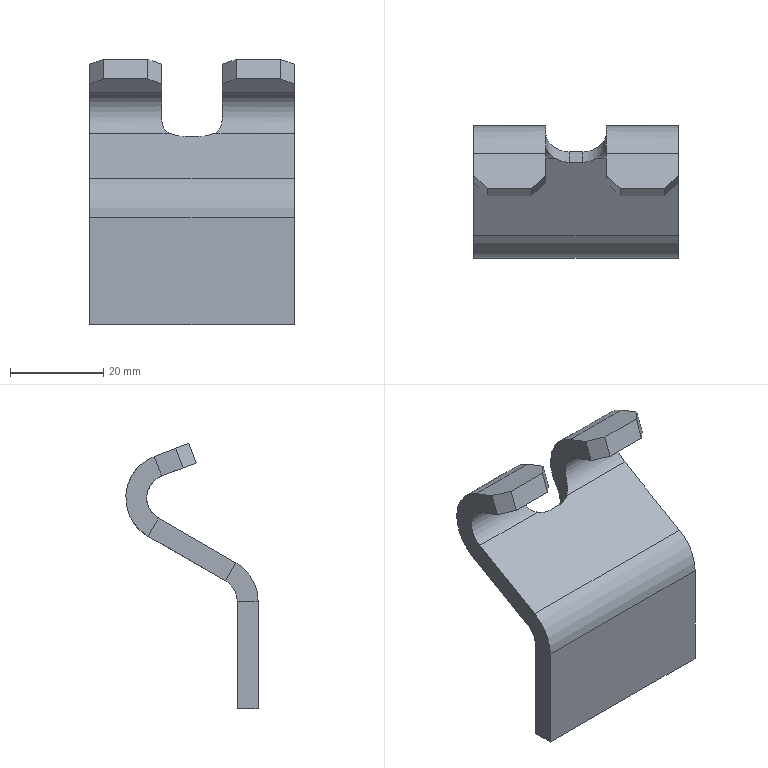Part | SolidWorks | features Chamfer 1, Fillet 1, FlatPattern 1, ICE 1, SMBaseFlange 1, SheetMetal 1 | 1 solid | 38 faces | box 44 x 28.417 x 57.001 mm | volume 13183 mm3 | plane 30 | cylinder 8 | commonest cylinder face diameters 10 x5 19 x3
STEP:
#1=CARTESIAN_POINT('',(23.5,9.499,-16.239));
#2=VERTEX_POINT('',#1);
#3=CARTESIAN_POINT('',(20.5,9.499,-16.239));
#4=VERTEX_POINT('',#3);
#5=CARTESIAN_POINT('',(28.5,9.499,-16.239));
#6=DIRECTION('',(-1.,0.,0.));
#7=VECTOR('',#6,1000.);
#8=LINE('',#5,#7);
#9=EDGE_CURVE('',#2,#4,#8,.T.);
#10=ORIENTED_EDGE('',*,*,#9,.F.);
#11=CARTESIAN_POINT('',(26.5,10.366,-15.739));
#12=VERTEX_POINT('',#11);
#13=CARTESIAN_POINT('',(23.5,13.83,-13.74));
#14=DIRECTION('',(0.,-0.4998,0.8661));
#15=DIRECTION('',(0.,0.8661,0.4998));
#16=AXIS2_PLACEMENT_3D('',#13,#14,#15);
#17=CIRCLE('',#16,5.);
#18=EDGE_CURVE('',#2,#12,#17,.T.);
#19=ORIENTED_EDGE('',*,*,#18,.T.);
#20=CARTESIAN_POINT('',(44.,10.366,-15.739));
#21=VERTEX_POINT('',#20);
#22=CARTESIAN_POINT('',(44.,10.366,-15.739));
#23=DIRECTION('',(-1.,0.,0.));
#24=VECTOR('',#23,1000.);
#25=LINE('',#22,#24);
#26=EDGE_CURVE('',#21,#12,#25,.T.);
#27=ORIENTED_EDGE('',*,*,#26,.F.);
#28=CARTESIAN_POINT('',(44.,-6.299,-25.356));
#29=VERTEX_POINT('',#28);
#30=CARTESIAN_POINT('',(44.,19.449,-10.498));
#31=DIRECTION('',(0.,-0.8661,-0.4998));
#32=VECTOR('',#31,1000.);
#33=LINE('',#30,#32);
#34=EDGE_CURVE('',#21,#29,#33,.T.);
#35=ORIENTED_EDGE('',*,*,#34,.T.);
#36=CARTESIAN_POINT('',(0.,-6.299,-25.356));
#37=VERTEX_POINT('',#36);
#38=CARTESIAN_POINT('',(44.,-6.299,-25.356));
#39=DIRECTION('',(-1.,0.,0.));
#40=VECTOR('',#39,1000.);
#41=LINE('',#38,#40);
#42=EDGE_CURVE('',#29,#37,#41,.T.);
#43=ORIENTED_EDGE('',*,*,#42,.T.);
#44=CARTESIAN_POINT('',(0.,10.366,-15.739));
#45=VERTEX_POINT('',#44);
#46=CARTESIAN_POINT('',(0.,19.449,-10.498));
#47=DIRECTION('',(0.,-0.8661,-0.4998));
#48=VECTOR('',#47,1000.);
#49=LINE('',#46,#48);
#50=EDGE_CURVE('',#45,#37,#49,.T.);
#51=ORIENTED_EDGE('',*,*,#50,.F.);
#52=CARTESIAN_POINT('',(17.5,10.366,-15.739));
#53=VERTEX_POINT('',#52);
#54=CARTESIAN_POINT('',(44.,10.366,-15.739));
#55=DIRECTION('',(-1.,0.,0.));
#56=VECTOR('',#55,1000.);
#57=LINE('',#54,#56);
#58=EDGE_CURVE('',#53,#45,#57,.T.);
#59=ORIENTED_EDGE('',*,*,#58,.F.);
#60=CARTESIAN_POINT('',(20.5,13.83,-13.74));
#61=DIRECTION('',(0.,-0.4998,0.8661));
#62=DIRECTION('',(0.,0.8661,0.4998));
#63=AXIS2_PLACEMENT_3D('',#60,#61,#62);
#64=CIRCLE('',#63,5.);
#65=EDGE_CURVE('',#53,#4,#64,.T.);
#66=ORIENTED_EDGE('',*,*,#65,.T.);
#67=EDGE_LOOP('',(#10,#19,#27,#35,#43,#51,#59,#66));
#68=FACE_OUTER_BOUND('',#67,.T.);
#69=CARTESIAN_POINT('',(44.,19.449,-10.498));
#70=DIRECTION('',(0.,0.4998,-0.8661));
#71=DIRECTION('',(0.,0.8661,0.4998));
#72=AXIS2_PLACEMENT_3D('',#69,#70,#71);
#73=PLANE('',#72);
#74=ADVANCED_FACE('',(#68),#73,.T.);
#75=ORIENTED_EDGE('',*,*,#26,.T.);
#76=CARTESIAN_POINT('',(28.5,13.389,-12.975));
#77=VERTEX_POINT('',#76);
#78=CARTESIAN_POINT('',(26.5,10.366,-15.739));
#79=CARTESIAN_POINT('',(26.82,10.574,-15.619));
#80=CARTESIAN_POINT('',(27.106,10.806,-15.475));
#81=CARTESIAN_POINT('',(27.483,11.183,-15.212));
#82=CARTESIAN_POINT('',(27.601,11.314,-15.116));
#83=CARTESIAN_POINT('',(27.815,11.579,-14.909));
#84=CARTESIAN_POINT('',(27.91,11.713,-14.8));
#85=CARTESIAN_POINT('',(28.081,11.982,-14.566));
#86=CARTESIAN_POINT('',(28.155,12.117,-14.443));
#87=CARTESIAN_POINT('',(28.283,12.386,-14.179));
#88=CARTESIAN_POINT('',(28.336,12.521,-14.04));
#89=CARTESIAN_POINT('',(28.461,12.912,-13.609));
#90=CARTESIAN_POINT('',(28.5,13.158,-13.303));
#91=CARTESIAN_POINT('',(28.5,13.389,-12.975));
#92=B_SPLINE_CURVE_WITH_KNOTS('',3,(#78,#79,#80,#81,#82,#83,#84,#85,#86,#87,#88,#89,#90,#91),.UNSPECIFIED.,.F.,.F.,(4,2,2,2,2,2,4),(0.,0.001185,0.001777,0.00237,0.002962,0.003555,0.00474),.UNSPECIFIED.);
#93=EDGE_CURVE('',#12,#77,#92,.T.);
#94=ORIENTED_EDGE('',*,*,#93,.T.);
#95=CARTESIAN_POINT('',(28.5,9.021,1.358));
#96=VERTEX_POINT('',#95);
#97=CARTESIAN_POINT('',(28.5,5.617,-7.511));
#98=DIRECTION('',(-1.,0.,0.));
#99=DIRECTION('',(0.,0.,-1.));
#100=AXIS2_PLACEMENT_3D('',#97,#98,#99);
#101=CIRCLE('',#100,9.5);
#102=EDGE_CURVE('',#96,#77,#101,.T.);
#103=ORIENTED_EDGE('',*,*,#102,.F.);
#104=CARTESIAN_POINT('',(44.,9.021,1.358));
#105=VERTEX_POINT('',#104);
#106=CARTESIAN_POINT('',(44.,9.021,1.358));
#107=DIRECTION('',(-1.,0.,0.));
#108=VECTOR('',#107,1000.);
#109=LINE('',#106,#108);
#110=EDGE_CURVE('',#105,#96,#109,.T.);
#111=ORIENTED_EDGE('',*,*,#110,.F.);
#112=CARTESIAN_POINT('',(44.,5.617,-7.511));
#113=DIRECTION('',(-1.,0.,0.));
#114=DIRECTION('',(0.,0.,-1.));
#115=AXIS2_PLACEMENT_3D('',#112,#113,#114);
#116=CIRCLE('',#115,9.5);
#117=EDGE_CURVE('',#105,#21,#116,.T.);
#118=ORIENTED_EDGE('',*,*,#117,.T.);
#119=EDGE_LOOP('',(#75,#94,#103,#111,#118));
#120=FACE_OUTER_BOUND('',#119,.T.);
#121=CARTESIAN_POINT('',(44.,5.617,-7.511));
#122=DIRECTION('',(-1.,0.,0.));
#123=DIRECTION('',(0.,0.,1.));
#124=AXIS2_PLACEMENT_3D('',#121,#122,#123);
#125=CYLINDRICAL_SURFACE('',#124,9.5);
#126=ADVANCED_FACE('',(#120),#125,.T.);
#127=CARTESIAN_POINT('',(15.5,9.021,1.358));
#128=VERTEX_POINT('',#127);
#129=CARTESIAN_POINT('',(0.,9.021,1.358));
#130=VERTEX_POINT('',#129);
#131=CARTESIAN_POINT('',(44.,9.021,1.358));
#132=DIRECTION('',(-1.,0.,0.));
#133=VECTOR('',#132,1000.);
#134=LINE('',#131,#133);
#135=EDGE_CURVE('',#128,#130,#134,.T.);
#136=ORIENTED_EDGE('',*,*,#135,.F.);
#137=CARTESIAN_POINT('',(15.5,13.389,-12.975));
#138=VERTEX_POINT('',#137);
#139=CARTESIAN_POINT('',(15.5,5.617,-7.511));
#140=DIRECTION('',(1.,0.,0.));
#141=DIRECTION('',(0.,0.,1.));
#142=AXIS2_PLACEMENT_3D('',#139,#140,#141);
#143=CIRCLE('',#142,9.5);
#144=EDGE_CURVE('',#138,#128,#143,.T.);
#145=ORIENTED_EDGE('',*,*,#144,.F.);
#146=CARTESIAN_POINT('',(15.5,13.389,-12.975));
#147=CARTESIAN_POINT('',(15.5,13.158,-13.303));
#148=CARTESIAN_POINT('',(15.539,12.912,-13.609));
#149=CARTESIAN_POINT('',(15.664,12.521,-14.04));
#150=CARTESIAN_POINT('',(15.717,12.387,-14.179));
#151=CARTESIAN_POINT('',(15.845,12.117,-14.442));
#152=CARTESIAN_POINT('',(15.919,11.982,-14.566));
#153=CARTESIAN_POINT('',(16.089,11.713,-14.8));
#154=CARTESIAN_POINT('',(16.185,11.579,-14.909));
#155=CARTESIAN_POINT('',(16.399,11.314,-15.115));
#156=CARTESIAN_POINT('',(16.517,11.183,-15.212));
#157=CARTESIAN_POINT('',(16.894,10.806,-15.475));
#158=CARTESIAN_POINT('',(17.18,10.574,-15.619));
#159=CARTESIAN_POINT('',(17.5,10.366,-15.739));
#160=B_SPLINE_CURVE_WITH_KNOTS('',3,(#146,#147,#148,#149,#150,#151,#152,#153,#154,#155,#156,#157,#158,#159),.UNSPECIFIED.,.F.,.F.,(4,2,2,2,2,2,4),(0.,0.001185,0.001777,0.00237,0.002962,0.003555,0.00474),.UNSPECIFIED.);
#161=EDGE_CURVE('',#138,#53,#160,.T.);
#162=ORIENTED_EDGE('',*,*,#161,.T.);
#163=ORIENTED_EDGE('',*,*,#58,.T.);
#164=CARTESIAN_POINT('',(0.,5.617,-7.511));
#165=DIRECTION('',(-1.,0.,0.));
#166=DIRECTION('',(0.,0.,-1.));
#167=AXIS2_PLACEMENT_3D('',#164,#165,#166);
#168=CIRCLE('',#167,9.5);
#169=EDGE_CURVE('',#130,#45,#168,.T.);
#170=ORIENTED_EDGE('',*,*,#169,.F.);
#171=EDGE_LOOP('',(#136,#145,#162,#163,#170));
#172=FACE_OUTER_BOUND('',#171,.T.);
#173=CARTESIAN_POINT('',(44.,5.617,-7.511));
#174=DIRECTION('',(-1.,0.,0.));
#175=DIRECTION('',(0.,0.,1.));
#176=AXIS2_PLACEMENT_3D('',#173,#174,#175);
#177=CYLINDRICAL_SURFACE('',#176,9.5);
#178=ADVANCED_FACE('',(#172),#177,.T.);
#179=CARTESIAN_POINT('',(41.,1.612,4.201));
#180=VERTEX_POINT('',#179);
#181=CARTESIAN_POINT('',(31.5,1.612,4.201));
#182=VERTEX_POINT('',#181);
#183=CARTESIAN_POINT('',(44.,1.612,4.201));
#184=DIRECTION('',(-1.,0.,0.));
#185=VECTOR('',#184,1000.);
#186=LINE('',#183,#185);
#187=EDGE_CURVE('',#180,#182,#186,.T.);
#188=ORIENTED_EDGE('',*,*,#187,.F.);
#189=CARTESIAN_POINT('',(44.,4.413,3.127));
#190=VERTEX_POINT('',#189);
#191=CARTESIAN_POINT('',(42.5,3.013,3.664));
#192=DIRECTION('',(0.7071,0.6602,-0.2533));
#193=VECTOR('',#192,1000.);
#194=LINE('',#191,#193);
#195=EDGE_CURVE('',#180,#190,#194,.T.);
#196=ORIENTED_EDGE('',*,*,#195,.T.);
#197=CARTESIAN_POINT('',(44.,1.612,4.201));
#198=DIRECTION('',(0.,0.9336,-0.3583));
#199=VECTOR('',#198,1000.);
#200=LINE('',#197,#199);
#201=EDGE_CURVE('',#190,#105,#200,.T.);
#202=ORIENTED_EDGE('',*,*,#201,.T.);
#203=ORIENTED_EDGE('',*,*,#110,.T.);
#204=CARTESIAN_POINT('',(28.5,4.413,3.127));
#205=VERTEX_POINT('',#204);
#206=CARTESIAN_POINT('',(28.5,1.612,4.201));
#207=DIRECTION('',(0.,0.9336,-0.3583));
#208=VECTOR('',#207,1000.);
#209=LINE('',#206,#208);
#210=EDGE_CURVE('',#205,#96,#209,.T.);
#211=ORIENTED_EDGE('',*,*,#210,.F.);
#212=CARTESIAN_POINT('',(37.75,-4.223,6.44));
#213=DIRECTION('',(0.7071,-0.6602,0.2533));
#214=VECTOR('',#213,1000.);
#215=LINE('',#212,#214);
#216=EDGE_CURVE('',#205,#182,#215,.T.);
#217=ORIENTED_EDGE('',*,*,#216,.T.);
#218=EDGE_LOOP('',(#188,#196,#202,#203,#211,#217));
#219=FACE_OUTER_BOUND('',#218,.T.);
#220=CARTESIAN_POINT('',(44.,1.612,4.201));
#221=DIRECTION('',(0.,0.3583,0.9336));
#222=DIRECTION('',(0.,-0.9336,0.3583));
#223=AXIS2_PLACEMENT_3D('',#220,#221,#222);
#224=PLANE('',#223);
#225=ADVANCED_FACE('',(#219),#224,.T.);
#226=CARTESIAN_POINT('',(12.5,1.612,4.201));
#227=VERTEX_POINT('',#226);
#228=CARTESIAN_POINT('',(3.,1.612,4.201));
#229=VERTEX_POINT('',#228);
#230=CARTESIAN_POINT('',(44.,1.612,4.201));
#231=DIRECTION('',(-1.,0.,0.));
#232=VECTOR('',#231,1000.);
#233=LINE('',#230,#232);
#234=EDGE_CURVE('',#227,#229,#233,.T.);
#235=ORIENTED_EDGE('',*,*,#234,.F.);
#236=CARTESIAN_POINT('',(15.5,4.413,3.127));
#237=VERTEX_POINT('',#236);
#238=CARTESIAN_POINT('',(28.25,16.317,-1.441));
#239=DIRECTION('',(0.7071,0.6602,-0.2533));
#240=VECTOR('',#239,1000.);
#241=LINE('',#238,#240);
#242=EDGE_CURVE('',#227,#237,#241,.T.);
#243=ORIENTED_EDGE('',*,*,#242,.T.);
#244=CARTESIAN_POINT('',(15.5,1.612,4.201));
#245=DIRECTION('',(0.,-0.9336,0.3583));
#246=VECTOR('',#245,1000.);
#247=LINE('',#244,#246);
#248=EDGE_CURVE('',#128,#237,#247,.T.);
#249=ORIENTED_EDGE('',*,*,#248,.F.);
#250=ORIENTED_EDGE('',*,*,#135,.T.);
#251=CARTESIAN_POINT('',(0.,4.413,3.127));
#252=VERTEX_POINT('',#251);
#253=CARTESIAN_POINT('',(0.,1.612,4.201));
#254=DIRECTION('',(0.,0.9336,-0.3583));
#255=VECTOR('',#254,1000.);
#256=LINE('',#253,#255);
#257=EDGE_CURVE('',#252,#130,#256,.T.);
#258=ORIENTED_EDGE('',*,*,#257,.F.);
#259=CARTESIAN_POINT('',(23.5,-17.527,11.545));
#260=DIRECTION('',(0.7071,-0.6602,0.2533));
#261=VECTOR('',#260,1000.);
#262=LINE('',#259,#261);
#263=EDGE_CURVE('',#252,#229,#262,.T.);
#264=ORIENTED_EDGE('',*,*,#263,.T.);
#265=EDGE_LOOP('',(#235,#243,#249,#250,#258,#264));
#266=FACE_OUTER_BOUND('',#265,.T.);
#267=CARTESIAN_POINT('',(44.,1.612,4.201));
#268=DIRECTION('',(0.,0.3583,0.9336));
#269=DIRECTION('',(0.,-0.9336,0.3583));
#270=AXIS2_PLACEMENT_3D('',#267,#268,#269);
#271=PLANE('',#270);
#272=ADVANCED_FACE('',(#266),#271,.T.);
#273=CARTESIAN_POINT('',(41.,0.,0.));
#274=VERTEX_POINT('',#273);
#275=CARTESIAN_POINT('',(31.5,0.,0.));
#276=VERTEX_POINT('',#275);
#277=CARTESIAN_POINT('',(44.,0.,0.));
#278=DIRECTION('',(-1.,0.,0.));
#279=VECTOR('',#278,1000.);
#280=LINE('',#277,#279);
#281=EDGE_CURVE('',#274,#276,#280,.T.);
#282=ORIENTED_EDGE('',*,*,#281,.F.);
#283=CARTESIAN_POINT('',(41.,0.,0.));
#284=DIRECTION('',(0.,0.3583,0.9336));
#285=VECTOR('',#284,1000.);
#286=LINE('',#283,#285);
#287=EDGE_CURVE('',#274,#180,#286,.T.);
#288=ORIENTED_EDGE('',*,*,#287,.T.);
#289=ORIENTED_EDGE('',*,*,#187,.T.);
#290=CARTESIAN_POINT('',(31.5,0.,0.));
#291=DIRECTION('',(0.,-0.3583,-0.9336));
#292=VECTOR('',#291,1000.);
#293=LINE('',#290,#292);
#294=EDGE_CURVE('',#182,#276,#293,.T.);
#295=ORIENTED_EDGE('',*,*,#294,.T.);
#296=EDGE_LOOP('',(#282,#288,#289,#295));
#297=FACE_OUTER_BOUND('',#296,.T.);
#298=CARTESIAN_POINT('',(44.,0.,0.));
#299=DIRECTION('',(0.,-0.9336,0.3583));
#300=DIRECTION('',(0.,-0.3583,-0.9336));
#301=AXIS2_PLACEMENT_3D('',#298,#299,#300);
#302=PLANE('',#301);
#303=ADVANCED_FACE('',(#297),#302,.T.);
#304=CARTESIAN_POINT('',(12.5,0.,0.));
#305=VERTEX_POINT('',#304);
#306=CARTESIAN_POINT('',(3.,0.,0.));
#307=VERTEX_POINT('',#306);
#308=CARTESIAN_POINT('',(44.,0.,0.));
#309=DIRECTION('',(-1.,0.,0.));
#310=VECTOR('',#309,1000.);
#311=LINE('',#308,#310);
#312=EDGE_CURVE('',#305,#307,#311,.T.);
#313=ORIENTED_EDGE('',*,*,#312,.F.);
#314=CARTESIAN_POINT('',(12.5,0.,0.));
#315=DIRECTION('',(0.,0.3583,0.9336));
#316=VECTOR('',#315,1000.);
#317=LINE('',#314,#316);
#318=EDGE_CURVE('',#305,#227,#317,.T.);
#319=ORIENTED_EDGE('',*,*,#318,.T.);
#320=ORIENTED_EDGE('',*,*,#234,.T.);
#321=CARTESIAN_POINT('',(3.,0.,0.));
#322=DIRECTION('',(0.,-0.3583,-0.9336));
#323=VECTOR('',#322,1000.);
#324=LINE('',#321,#323);
#325=EDGE_CURVE('',#229,#307,#324,.T.);
#326=ORIENTED_EDGE('',*,*,#325,.T.);
#327=EDGE_LOOP('',(#313,#319,#320,#326));
#328=FACE_OUTER_BOUND('',#327,.T.);
#329=CARTESIAN_POINT('',(44.,0.,0.));
#330=DIRECTION('',(0.,-0.9336,0.3583));
#331=DIRECTION('',(0.,-0.3583,-0.9336));
#332=AXIS2_PLACEMENT_3D('',#329,#330,#331);
#333=PLANE('',#332);
#334=ADVANCED_FACE('',(#328),#333,.T.);
#335=CARTESIAN_POINT('',(44.,2.801,-1.075));
#336=VERTEX_POINT('',#335);
#337=CARTESIAN_POINT('',(44.,7.409,-2.843));
#338=VERTEX_POINT('',#337);
#339=CARTESIAN_POINT('',(44.,0.,0.));
#340=DIRECTION('',(0.,0.9336,-0.3583));
#341=VECTOR('',#340,1000.);
#342=LINE('',#339,#341);
#343=EDGE_CURVE('',#336,#338,#342,.T.);
#344=ORIENTED_EDGE('',*,*,#343,.F.);
#345=CARTESIAN_POINT('',(41.,0.,0.));
#346=DIRECTION('',(-0.7071,-0.6602,0.2533));
#347=VECTOR('',#346,1000.);
#348=LINE('',#345,#347);
#349=EDGE_CURVE('',#336,#274,#348,.T.);
#350=ORIENTED_EDGE('',*,*,#349,.T.);
#351=ORIENTED_EDGE('',*,*,#281,.T.);
#352=CARTESIAN_POINT('',(28.5,2.801,-1.075));
#353=VERTEX_POINT('',#352);
#354=CARTESIAN_POINT('',(31.5,0.,0.));
#355=DIRECTION('',(-0.7071,0.6602,-0.2533));
#356=VECTOR('',#355,1000.);
#357=LINE('',#354,#356);
#358=EDGE_CURVE('',#276,#353,#357,.T.);
#359=ORIENTED_EDGE('',*,*,#358,.T.);
#360=CARTESIAN_POINT('',(28.5,7.409,-2.843));
#361=VERTEX_POINT('',#360);
#362=CARTESIAN_POINT('',(28.5,0.,0.));
#363=DIRECTION('',(0.,0.9336,-0.3583));
#364=VECTOR('',#363,1000.);
#365=LINE('',#362,#364);
#366=EDGE_CURVE('',#353,#361,#365,.T.);
#367=ORIENTED_EDGE('',*,*,#366,.T.);
#368=CARTESIAN_POINT('',(44.,7.409,-2.843));
#369=DIRECTION('',(-1.,0.,0.));
#370=VECTOR('',#369,1000.);
#371=LINE('',#368,#370);
#372=EDGE_CURVE('',#338,#361,#371,.T.);
#373=ORIENTED_EDGE('',*,*,#372,.F.);
#374=EDGE_LOOP('',(#344,#350,#351,#359,#367,#373));
#375=FACE_OUTER_BOUND('',#374,.T.);
#376=CARTESIAN_POINT('',(44.,0.,0.));
#377=DIRECTION('',(0.,0.3583,0.9336));
#378=DIRECTION('',(0.,-0.9336,0.3583));
#379=AXIS2_PLACEMENT_3D('',#376,#377,#378);
#380=PLANE('',#379);
#381=ADVANCED_FACE('',(#375),#380,.F.);
#382=CARTESIAN_POINT('',(15.5,7.409,-2.843));
#383=VERTEX_POINT('',#382);
#384=CARTESIAN_POINT('',(15.5,2.801,-1.075));
#385=VERTEX_POINT('',#384);
#386=CARTESIAN_POINT('',(15.5,0.,0.));
#387=DIRECTION('',(0.,-0.9336,0.3583));
#388=VECTOR('',#387,1000.);
#389=LINE('',#386,#388);
#390=EDGE_CURVE('',#383,#385,#389,.T.);
#391=ORIENTED_EDGE('',*,*,#390,.T.);
#392=CARTESIAN_POINT('',(15.5,2.801,-1.075));
#393=DIRECTION('',(-0.7071,-0.6602,0.2533));
#394=VECTOR('',#393,1000.);
#395=LINE('',#392,#394);
#396=EDGE_CURVE('',#385,#305,#395,.T.);
#397=ORIENTED_EDGE('',*,*,#396,.T.);
#398=ORIENTED_EDGE('',*,*,#312,.T.);
#399=CARTESIAN_POINT('',(0.,2.801,-1.075));
#400=VERTEX_POINT('',#399);
#401=CARTESIAN_POINT('',(0.,2.801,-1.075));
#402=DIRECTION('',(-0.7071,0.6602,-0.2533));
#403=VECTOR('',#402,1000.);
#404=LINE('',#401,#403);
#405=EDGE_CURVE('',#307,#400,#404,.T.);
#406=ORIENTED_EDGE('',*,*,#405,.T.);
#407=CARTESIAN_POINT('',(0.,7.409,-2.843));
#408=VERTEX_POINT('',#407);
#409=CARTESIAN_POINT('',(0.,0.,0.));
#410=DIRECTION('',(0.,0.9336,-0.3583));
#411=VECTOR('',#410,1000.);
#412=LINE('',#409,#411);
#413=EDGE_CURVE('',#400,#408,#412,.T.);
#414=ORIENTED_EDGE('',*,*,#413,.T.);
#415=CARTESIAN_POINT('',(44.,7.409,-2.843));
#416=DIRECTION('',(-1.,0.,0.));
#417=VECTOR('',#416,1000.);
#418=LINE('',#415,#417);
#419=EDGE_CURVE('',#383,#408,#418,.T.);
#420=ORIENTED_EDGE('',*,*,#419,.F.);
#421=EDGE_LOOP('',(#391,#397,#398,#406,#414,#420));
#422=FACE_OUTER_BOUND('',#421,.T.);
#423=CARTESIAN_POINT('',(44.,0.,0.));
#424=DIRECTION('',(0.,0.3583,0.9336));
#425=DIRECTION('',(0.,-0.9336,0.3583));
#426=AXIS2_PLACEMENT_3D('',#423,#424,#425);
#427=PLANE('',#426);
#428=ADVANCED_FACE('',(#422),#427,.F.);
#429=CARTESIAN_POINT('',(28.5,10.581,-8.11));
#430=VERTEX_POINT('',#429);
#431=CARTESIAN_POINT('',(28.5,5.617,-7.511));
#432=DIRECTION('',(-1.,0.,0.));
#433=DIRECTION('',(0.,0.,1.));
#434=AXIS2_PLACEMENT_3D('',#431,#432,#433);
#435=CIRCLE('',#434,5.);
#436=EDGE_CURVE('',#361,#430,#435,.T.);
#437=ORIENTED_EDGE('',*,*,#436,.T.);
#438=CARTESIAN_POINT('',(26.5,8.116,-11.842));
#439=VERTEX_POINT('',#438);
#440=CARTESIAN_POINT('',(28.5,10.581,-8.11));
#441=CARTESIAN_POINT('',(28.5,10.528,-8.548));
#442=CARTESIAN_POINT('',(28.48,10.42,-8.97));
#443=CARTESIAN_POINT('',(28.384,10.176,-9.577));
#444=CARTESIAN_POINT('',(28.342,10.082,-9.772));
#445=CARTESIAN_POINT('',(28.232,9.876,-10.139));
#446=CARTESIAN_POINT('',(28.165,9.763,-10.313));
#447=CARTESIAN_POINT('',(28.003,9.521,-10.641));
#448=CARTESIAN_POINT('',(27.907,9.393,-10.795));
#449=CARTESIAN_POINT('',(27.691,9.133,-11.072));
#450=CARTESIAN_POINT('',(27.571,9.001,-11.197));
#451=CARTESIAN_POINT('',(27.303,8.736,-11.423));
#452=CARTESIAN_POINT('',(27.155,8.604,-11.524));
#453=CARTESIAN_POINT('',(26.843,8.352,-11.699));
#454=CARTESIAN_POINT('',(26.677,8.231,-11.775));
#455=CARTESIAN_POINT('',(26.5,8.116,-11.842));
#456=B_SPLINE_CURVE_WITH_KNOTS('',3,(#440,#441,#442,#443,#444,#445,#446,#447,#448,#449,#450,#451,#452,#453,#454,#455),.UNSPECIFIED.,.F.,.F.,(4,2,2,2,2,2,2,4),(0.,0.001308,0.001962,0.002617,0.003271,0.003925,0.004579,0.005233),.UNSPECIFIED.);
#457=EDGE_CURVE('',#430,#439,#456,.T.);
#458=ORIENTED_EDGE('',*,*,#457,.T.);
#459=CARTESIAN_POINT('',(44.,8.116,-11.842));
#460=VERTEX_POINT('',#459);
#461=CARTESIAN_POINT('',(44.,8.116,-11.842));
#462=DIRECTION('',(-1.,0.,0.));
#463=VECTOR('',#462,1000.);
#464=LINE('',#461,#463);
#465=EDGE_CURVE('',#460,#439,#464,.T.);
#466=ORIENTED_EDGE('',*,*,#465,.F.);
#467=CARTESIAN_POINT('',(44.,5.617,-7.511));
#468=DIRECTION('',(-1.,0.,0.));
#469=DIRECTION('',(0.,0.,-1.));
#470=AXIS2_PLACEMENT_3D('',#467,#468,#469);
#471=CIRCLE('',#470,5.);
#472=EDGE_CURVE('',#338,#460,#471,.T.);
#473=ORIENTED_EDGE('',*,*,#472,.F.);
#474=ORIENTED_EDGE('',*,*,#372,.T.);
#475=EDGE_LOOP('',(#437,#458,#466,#473,#474));
#476=FACE_OUTER_BOUND('',#475,.T.);
#477=CARTESIAN_POINT('',(44.,5.617,-7.511));
#478=DIRECTION('',(-1.,0.,0.));
#479=DIRECTION('',(0.,0.,1.));
#480=AXIS2_PLACEMENT_3D('',#477,#478,#479);
#481=CYLINDRICAL_SURFACE('',#480,5.);
#482=ADVANCED_FACE('',(#476),#481,.F.);
#483=CARTESIAN_POINT('',(17.5,8.116,-11.842));
#484=VERTEX_POINT('',#483);
#485=CARTESIAN_POINT('',(0.,8.116,-11.842));
#486=VERTEX_POINT('',#485);
#487=CARTESIAN_POINT('',(44.,8.116,-11.842));
#488=DIRECTION('',(-1.,0.,0.));
#489=VECTOR('',#488,1000.);
#490=LINE('',#487,#489);
#491=EDGE_CURVE('',#484,#486,#490,.T.);
#492=ORIENTED_EDGE('',*,*,#491,.F.);
#493=CARTESIAN_POINT('',(15.5,10.581,-8.11));
#494=VERTEX_POINT('',#493);
#495=CARTESIAN_POINT('',(17.5,8.116,-11.842));
#496=CARTESIAN_POINT('',(17.147,8.346,-11.709));
#497=CARTESIAN_POINT('',(16.836,8.6,-11.539));
#498=CARTESIAN_POINT('',(16.432,8.998,-11.199));
#499=CARTESIAN_POINT('',(16.31,9.131,-11.073));
#500=CARTESIAN_POINT('',(16.095,9.39,-10.798));
#501=CARTESIAN_POINT('',(16.001,9.517,-10.647));
#502=CARTESIAN_POINT('',(15.837,9.759,-10.32));
#503=CARTESIAN_POINT('',(15.769,9.874,-10.143));
#504=CARTESIAN_POINT('',(15.659,10.081,-9.774));
#505=CARTESIAN_POINT('',(15.617,10.174,-9.581));
#506=CARTESIAN_POINT('',(15.553,10.336,-9.178));
#507=CARTESIAN_POINT('',(15.532,10.405,-8.969));
#508=CARTESIAN_POINT('',(15.505,10.514,-8.545));
#509=CARTESIAN_POINT('',(15.5,10.555,-8.329));
#510=CARTESIAN_POINT('',(15.5,10.581,-8.11));
#511=B_SPLINE_CURVE_WITH_KNOTS('',3,(#495,#496,#497,#498,#499,#500,#501,#502,#503,#504,#505,#506,#507,#508,#509,#510),.UNSPECIFIED.,.F.,.F.,(4,2,2,2,2,2,2,4),(0.,0.001308,0.001962,0.002617,0.003271,0.003925,0.004579,0.005233),.UNSPECIFIED.);
#512=EDGE_CURVE('',#484,#494,#511,.T.);
#513=ORIENTED_EDGE('',*,*,#512,.T.);
#514=CARTESIAN_POINT('',(15.5,5.617,-7.511));
#515=DIRECTION('',(1.,0.,0.));
#516=DIRECTION('',(0.,0.,1.));
#517=AXIS2_PLACEMENT_3D('',#514,#515,#516);
#518=CIRCLE('',#517,5.);
#519=EDGE_CURVE('',#494,#383,#518,.T.);
#520=ORIENTED_EDGE('',*,*,#519,.T.);
#521=ORIENTED_EDGE('',*,*,#419,.T.);
#522=CARTESIAN_POINT('',(0.,5.617,-7.511));
#523=DIRECTION('',(-1.,0.,0.));
#524=DIRECTION('',(0.,0.,-1.));
#525=AXIS2_PLACEMENT_3D('',#522,#523,#524);
#526=CIRCLE('',#525,5.);
#527=EDGE_CURVE('',#408,#486,#526,.T.);
#528=ORIENTED_EDGE('',*,*,#527,.T.);
#529=EDGE_LOOP('',(#492,#513,#520,#521,#528));
#530=FACE_OUTER_BOUND('',#529,.T.);
#531=CARTESIAN_POINT('',(44.,5.617,-7.511));
#532=DIRECTION('',(-1.,0.,0.));
#533=DIRECTION('',(0.,0.,1.));
#534=AXIS2_PLACEMENT_3D('',#531,#532,#533);
#535=CYLINDRICAL_SURFACE('',#534,5.);
#536=ADVANCED_FACE('',(#530),#535,.F.);
#537=ORIENTED_EDGE('',*,*,#465,.T.);
#538=CARTESIAN_POINT('',(23.5,7.25,-12.341));
#539=VERTEX_POINT('',#538);
#540=CARTESIAN_POINT('',(23.5,11.581,-9.842));
#541=DIRECTION('',(0.,0.4998,-0.8661));
#542=DIRECTION('',(0.,0.8661,0.4998));
#543=AXIS2_PLACEMENT_3D('',#540,#541,#542);
#544=CIRCLE('',#543,5.);
#545=EDGE_CURVE('',#439,#539,#544,.T.);
#546=ORIENTED_EDGE('',*,*,#545,.T.);
#547=CARTESIAN_POINT('',(20.5,7.25,-12.341));
#548=VERTEX_POINT('',#547);
#549=CARTESIAN_POINT('',(44.,7.25,-12.341));
#550=DIRECTION('',(-1.,0.,0.));
#551=VECTOR('',#550,1000.);
#552=LINE('',#549,#551);
#553=EDGE_CURVE('',#539,#548,#552,.T.);
#554=ORIENTED_EDGE('',*,*,#553,.T.);
#555=CARTESIAN_POINT('',(20.5,11.581,-9.842));
#556=DIRECTION('',(0.,0.4998,-0.8661));
#557=DIRECTION('',(0.,0.8661,0.4998));
#558=AXIS2_PLACEMENT_3D('',#555,#556,#557);
#559=CIRCLE('',#558,5.);
#560=EDGE_CURVE('',#548,#484,#559,.T.);
#561=ORIENTED_EDGE('',*,*,#560,.T.);
#562=ORIENTED_EDGE('',*,*,#491,.T.);
#563=CARTESIAN_POINT('',(0.,-8.548,-21.458));
#564=VERTEX_POINT('',#563);
#565=CARTESIAN_POINT('',(0.,17.2,-6.6));
#566=DIRECTION('',(0.,-0.8661,-0.4998));
#567=VECTOR('',#566,1000.);
#568=LINE('',#565,#567);
#569=EDGE_CURVE('',#486,#564,#568,.T.);
#570=ORIENTED_EDGE('',*,*,#569,.T.);
#571=CARTESIAN_POINT('',(44.,-8.548,-21.458));
#572=VERTEX_POINT('',#571);
#573=CARTESIAN_POINT('',(44.,-8.548,-21.458));
#574=DIRECTION('',(-1.,0.,0.));
#575=VECTOR('',#574,1000.);
#576=LINE('',#573,#575);
#577=EDGE_CURVE('',#572,#564,#576,.T.);
#578=ORIENTED_EDGE('',*,*,#577,.F.);
#579=CARTESIAN_POINT('',(44.,17.2,-6.6));
#580=DIRECTION('',(0.,-0.8661,-0.4998));
#581=VECTOR('',#580,1000.);
#582=LINE('',#579,#581);
#583=EDGE_CURVE('',#460,#572,#582,.T.);
#584=ORIENTED_EDGE('',*,*,#583,.F.);
#585=EDGE_LOOP('',(#537,#546,#554,#561,#562,#570,#578,#584));
#586=FACE_OUTER_BOUND('',#585,.T.);
#587=CARTESIAN_POINT('',(44.,17.2,-6.6));
#588=DIRECTION('',(0.,0.4998,-0.8661));
#589=DIRECTION('',(0.,0.8661,0.4998));
#590=AXIS2_PLACEMENT_3D('',#587,#588,#589);
#591=PLANE('',#590);
#592=ADVANCED_FACE('',(#586),#591,.F.);
#593=CARTESIAN_POINT('',(44.,7.409,-2.843));
#594=DIRECTION('',(0.,0.3583,0.9336));
#595=VECTOR('',#594,1000.);
#596=LINE('',#593,#595);
#597=EDGE_CURVE('',#338,#105,#596,.T.);
#598=ORIENTED_EDGE('',*,*,#597,.F.);
#599=ORIENTED_EDGE('',*,*,#472,.T.);
#600=CARTESIAN_POINT('',(44.,10.366,-15.739));
#601=DIRECTION('',(0.,-0.4998,0.8661));
#602=VECTOR('',#601,1000.);
#603=LINE('',#600,#602);
#604=EDGE_CURVE('',#21,#460,#603,.T.);
#605=ORIENTED_EDGE('',*,*,#604,.F.);
#606=ORIENTED_EDGE('',*,*,#117,.F.);
#607=EDGE_LOOP('',(#598,#599,#605,#606));
#608=FACE_OUTER_BOUND('',#607,.T.);
#609=CARTESIAN_POINT('',(44.,7.409,-2.843));
#610=DIRECTION('',(1.,0.,0.));
#611=DIRECTION('',(0.,0.,-1.));
#612=AXIS2_PLACEMENT_3D('',#609,#610,#611);
#613=PLANE('',#612);
#614=ADVANCED_FACE('',(#608),#613,.T.);
#615=ORIENTED_EDGE('',*,*,#201,.F.);
#616=CARTESIAN_POINT('',(44.,-1.133,-11.327));
#617=DIRECTION('',(0.,-0.3583,-0.9336));
#618=VECTOR('',#617,1000.);
#619=LINE('',#616,#618);
#620=EDGE_CURVE('',#190,#336,#619,.T.);
#621=ORIENTED_EDGE('',*,*,#620,.T.);
#622=ORIENTED_EDGE('',*,*,#343,.T.);
#623=ORIENTED_EDGE('',*,*,#597,.T.);
#624=EDGE_LOOP('',(#615,#621,#622,#623));
#625=FACE_OUTER_BOUND('',#624,.T.);
#626=CARTESIAN_POINT('',(44.,10.366,-15.739));
#627=DIRECTION('',(1.,0.,0.));
#628=DIRECTION('',(0.,0.,-1.));
#629=AXIS2_PLACEMENT_3D('',#626,#627,#628);
#630=PLANE('',#629);
#631=ADVANCED_FACE('',(#625),#630,.T.);
#632=CARTESIAN_POINT('',(0.,8.116,-11.842));
#633=DIRECTION('',(0.,0.4998,-0.8661));
#634=VECTOR('',#633,1000.);
#635=LINE('',#632,#634);
#636=EDGE_CURVE('',#486,#45,#635,.T.);
#637=ORIENTED_EDGE('',*,*,#636,.F.);
#638=ORIENTED_EDGE('',*,*,#527,.F.);
#639=CARTESIAN_POINT('',(0.,9.021,1.358));
#640=DIRECTION('',(0.,-0.3583,-0.9336));
#641=VECTOR('',#640,1000.);
#642=LINE('',#639,#641);
#643=EDGE_CURVE('',#130,#408,#642,.T.);
#644=ORIENTED_EDGE('',*,*,#643,.F.);
#645=ORIENTED_EDGE('',*,*,#169,.T.);
#646=EDGE_LOOP('',(#637,#638,#644,#645));
#647=FACE_OUTER_BOUND('',#646,.T.);
#648=CARTESIAN_POINT('',(0.,8.116,-11.842));
#649=DIRECTION('',(-1.,0.,0.));
#650=DIRECTION('',(0.,0.,1.));
#651=AXIS2_PLACEMENT_3D('',#648,#649,#650);
#652=PLANE('',#651);
#653=ADVANCED_FACE('',(#647),#652,.T.);
#654=ORIENTED_EDGE('',*,*,#569,.F.);
#655=ORIENTED_EDGE('',*,*,#636,.T.);
#656=ORIENTED_EDGE('',*,*,#50,.T.);
#657=CARTESIAN_POINT('',(0.,-6.299,-25.356));
#658=DIRECTION('',(0.,-0.4998,0.8661));
#659=VECTOR('',#658,1000.);
#660=LINE('',#657,#659);
#661=EDGE_CURVE('',#37,#564,#660,.T.);
#662=ORIENTED_EDGE('',*,*,#661,.T.);
#663=EDGE_LOOP('',(#654,#655,#656,#662));
#664=FACE_OUTER_BOUND('',#663,.T.);
#665=CARTESIAN_POINT('',(0.,9.021,1.358));
#666=DIRECTION('',(-1.,0.,0.));
#667=DIRECTION('',(0.,0.,1.));
#668=AXIS2_PLACEMENT_3D('',#665,#666,#667);
#669=PLANE('',#668);
#670=ADVANCED_FACE('',(#664),#669,.T.);
#671=CARTESIAN_POINT('',(44.,-8.548,-21.458));
#672=DIRECTION('',(0.,0.4998,-0.8661));
#673=VECTOR('',#672,1000.);
#674=LINE('',#671,#673);
#675=EDGE_CURVE('',#572,#29,#674,.T.);
#676=ORIENTED_EDGE('',*,*,#675,.F.);
#677=CARTESIAN_POINT('',(44.,-13.3,-29.686));
#678=VERTEX_POINT('',#677);
#679=CARTESIAN_POINT('',(44.,-3.8,-29.686));
#680=DIRECTION('',(1.,0.,0.));
#681=DIRECTION('',(0.,0.,1.));
#682=AXIS2_PLACEMENT_3D('',#679,#680,#681);
#683=CIRCLE('',#682,9.5);
#684=EDGE_CURVE('',#572,#678,#683,.T.);
#685=ORIENTED_EDGE('',*,*,#684,.T.);
#686=CARTESIAN_POINT('',(44.,-8.8,-29.686));
#687=VERTEX_POINT('',#686);
#688=CARTESIAN_POINT('',(44.,-8.8,-29.686));
#689=DIRECTION('',(0.,-1.,0.));
#690=VECTOR('',#689,1000.);
#691=LINE('',#688,#690);
#692=EDGE_CURVE('',#687,#678,#691,.T.);
#693=ORIENTED_EDGE('',*,*,#692,.F.);
#694=CARTESIAN_POINT('',(44.,-3.8,-29.686));
#695=DIRECTION('',(1.,0.,0.));
#696=DIRECTION('',(0.,0.,-1.));
#697=AXIS2_PLACEMENT_3D('',#694,#695,#696);
#698=CIRCLE('',#697,5.);
#699=EDGE_CURVE('',#29,#687,#698,.T.);
#700=ORIENTED_EDGE('',*,*,#699,.F.);
#701=EDGE_LOOP('',(#676,#685,#693,#700));
#702=FACE_OUTER_BOUND('',#701,.T.);
#703=CARTESIAN_POINT('',(44.,-8.548,-21.458));
#704=DIRECTION('',(1.,0.,0.));
#705=DIRECTION('',(0.,0.,-1.));
#706=AXIS2_PLACEMENT_3D('',#703,#704,#705);
#707=PLANE('',#706);
#708=ADVANCED_FACE('',(#702),#707,.T.);
#709=ORIENTED_EDGE('',*,*,#583,.T.);
#710=ORIENTED_EDGE('',*,*,#675,.T.);
#711=ORIENTED_EDGE('',*,*,#34,.F.);
#712=ORIENTED_EDGE('',*,*,#604,.T.);
#713=EDGE_LOOP('',(#709,#710,#711,#712));
#714=FACE_OUTER_BOUND('',#713,.T.);
#715=CARTESIAN_POINT('',(44.,-8.8,-29.686));
#716=DIRECTION('',(1.,0.,0.));
#717=DIRECTION('',(0.,0.,-1.));
#718=AXIS2_PLACEMENT_3D('',#715,#716,#717);
#719=PLANE('',#718);
#720=ADVANCED_FACE('',(#714),#719,.T.);
#721=CARTESIAN_POINT('',(0.,-13.3,-29.686));
#722=VERTEX_POINT('',#721);
#723=CARTESIAN_POINT('',(0.,-8.8,-29.686));
#724=VERTEX_POINT('',#723);
#725=CARTESIAN_POINT('',(0.,-13.3,-29.686));
#726=DIRECTION('',(0.,1.,0.));
#727=VECTOR('',#726,1000.);
#728=LINE('',#725,#727);
#729=EDGE_CURVE('',#722,#724,#728,.T.);
#730=ORIENTED_EDGE('',*,*,#729,.F.);
#731=CARTESIAN_POINT('',(0.,-3.8,-29.686));
#732=DIRECTION('',(1.,0.,0.));
#733=DIRECTION('',(0.,0.,1.));
#734=AXIS2_PLACEMENT_3D('',#731,#732,#733);
#735=CIRCLE('',#734,9.5);
#736=EDGE_CURVE('',#564,#722,#735,.T.);
#737=ORIENTED_EDGE('',*,*,#736,.F.);
#738=ORIENTED_EDGE('',*,*,#661,.F.);
#739=CARTESIAN_POINT('',(0.,-3.8,-29.686));
#740=DIRECTION('',(1.,0.,0.));
#741=DIRECTION('',(0.,0.,-1.));
#742=AXIS2_PLACEMENT_3D('',#739,#740,#741);
#743=CIRCLE('',#742,5.);
#744=EDGE_CURVE('',#37,#724,#743,.T.);
#745=ORIENTED_EDGE('',*,*,#744,.T.);
#746=EDGE_LOOP('',(#730,#737,#738,#745));
#747=FACE_OUTER_BOUND('',#746,.T.);
#748=CARTESIAN_POINT('',(0.,-13.3,-29.686));
#749=DIRECTION('',(-1.,0.,0.));
#750=DIRECTION('',(0.,0.,1.));
#751=AXIS2_PLACEMENT_3D('',#748,#749,#750);
#752=PLANE('',#751);
#753=ADVANCED_FACE('',(#747),#752,.T.);
#754=CARTESIAN_POINT('',(0.,-13.3,-52.8));
#755=VERTEX_POINT('',#754);
#756=CARTESIAN_POINT('',(0.,-13.3,-24.2));
#757=DIRECTION('',(0.,0.,-1.));
#758=VECTOR('',#757,1000.);
#759=LINE('',#756,#758);
#760=EDGE_CURVE('',#722,#755,#759,.T.);
#761=ORIENTED_EDGE('',*,*,#760,.F.);
#762=ORIENTED_EDGE('',*,*,#729,.T.);
#763=CARTESIAN_POINT('',(0.,-8.8,-52.8));
#764=VERTEX_POINT('',#763);
#765=CARTESIAN_POINT('',(0.,-8.8,-24.2));
#766=DIRECTION('',(0.,0.,-1.));
#767=VECTOR('',#766,1000.);
#768=LINE('',#765,#767);
#769=EDGE_CURVE('',#724,#764,#768,.T.);
#770=ORIENTED_EDGE('',*,*,#769,.T.);
#771=CARTESIAN_POINT('',(0.,-8.8,-52.8));
#772=DIRECTION('',(0.,-1.,0.));
#773=VECTOR('',#772,1000.);
#774=LINE('',#771,#773);
#775=EDGE_CURVE('',#764,#755,#774,.T.);
#776=ORIENTED_EDGE('',*,*,#775,.T.);
#777=EDGE_LOOP('',(#761,#762,#770,#776));
#778=FACE_OUTER_BOUND('',#777,.T.);
#779=CARTESIAN_POINT('',(0.,-6.299,-25.356));
#780=DIRECTION('',(-1.,0.,0.));
#781=DIRECTION('',(0.,0.,1.));
#782=AXIS2_PLACEMENT_3D('',#779,#780,#781);
#783=PLANE('',#782);
#784=ADVANCED_FACE('',(#778),#783,.T.);
#785=ORIENTED_EDGE('',*,*,#760,.T.);
#786=CARTESIAN_POINT('',(44.,-13.3,-52.8));
#787=VERTEX_POINT('',#786);
#788=CARTESIAN_POINT('',(44.,-13.3,-52.8));
#789=DIRECTION('',(-1.,0.,0.));
#790=VECTOR('',#789,1000.);
#791=LINE('',#788,#790);
#792=EDGE_CURVE('',#787,#755,#791,.T.);
#793=ORIENTED_EDGE('',*,*,#792,.F.);
#794=CARTESIAN_POINT('',(44.,-13.3,-24.2));
#795=DIRECTION('',(0.,0.,-1.));
#796=VECTOR('',#795,1000.);
#797=LINE('',#794,#796);
#798=EDGE_CURVE('',#678,#787,#797,.T.);
#799=ORIENTED_EDGE('',*,*,#798,.F.);
#800=CARTESIAN_POINT('',(44.,-13.3,-29.686));
#801=DIRECTION('',(-1.,0.,0.));
#802=VECTOR('',#801,1000.);
#803=LINE('',#800,#802);
#804=EDGE_CURVE('',#678,#722,#803,.T.);
#805=ORIENTED_EDGE('',*,*,#804,.T.);
#806=EDGE_LOOP('',(#785,#793,#799,#805));
#807=FACE_OUTER_BOUND('',#806,.T.);
#808=CARTESIAN_POINT('',(44.,-13.3,-24.2));
#809=DIRECTION('',(0.,1.,0.));
#810=DIRECTION('',(0.,0.,1.));
#811=AXIS2_PLACEMENT_3D('',#808,#809,#810);
#812=PLANE('',#811);
#813=ADVANCED_FACE('',(#807),#812,.F.);
#814=ORIENTED_EDGE('',*,*,#775,.F.);
#815=CARTESIAN_POINT('',(44.,-8.8,-52.8));
#816=VERTEX_POINT('',#815);
#817=CARTESIAN_POINT('',(44.,-8.8,-52.8));
#818=DIRECTION('',(-1.,0.,0.));
#819=VECTOR('',#818,1000.);
#820=LINE('',#817,#819);
#821=EDGE_CURVE('',#816,#764,#820,.T.);
#822=ORIENTED_EDGE('',*,*,#821,.F.);
#823=CARTESIAN_POINT('',(44.,-8.8,-52.8));
#824=DIRECTION('',(0.,-1.,0.));
#825=VECTOR('',#824,1000.);
#826=LINE('',#823,#825);
#827=EDGE_CURVE('',#816,#787,#826,.T.);
#828=ORIENTED_EDGE('',*,*,#827,.T.);
#829=ORIENTED_EDGE('',*,*,#792,.T.);
#830=EDGE_LOOP('',(#814,#822,#828,#829));
#831=FACE_OUTER_BOUND('',#830,.T.);
#832=CARTESIAN_POINT('',(44.,-8.8,-52.8));
#833=DIRECTION('',(0.,0.,-1.));
#834=DIRECTION('',(-1.,0.,0.));
#835=AXIS2_PLACEMENT_3D('',#832,#833,#834);
#836=PLANE('',#835);
#837=ADVANCED_FACE('',(#831),#836,.T.);
#838=ORIENTED_EDGE('',*,*,#769,.F.);
#839=CARTESIAN_POINT('',(44.,-8.8,-29.686));
#840=DIRECTION('',(-1.,0.,0.));
#841=VECTOR('',#840,1000.);
#842=LINE('',#839,#841);
#843=EDGE_CURVE('',#687,#724,#842,.T.);
#844=ORIENTED_EDGE('',*,*,#843,.F.);
#845=CARTESIAN_POINT('',(44.,-8.8,-24.2));
#846=DIRECTION('',(0.,0.,-1.));
#847=VECTOR('',#846,1000.);
#848=LINE('',#845,#847);
#849=EDGE_CURVE('',#687,#816,#848,.T.);
#850=ORIENTED_EDGE('',*,*,#849,.T.);
#851=ORIENTED_EDGE('',*,*,#821,.T.);
#852=EDGE_LOOP('',(#838,#844,#850,#851));
#853=FACE_OUTER_BOUND('',#852,.T.);
#854=CARTESIAN_POINT('',(44.,-8.8,-24.2));
#855=DIRECTION('',(0.,1.,0.));
#856=DIRECTION('',(0.,0.,1.));
#857=AXIS2_PLACEMENT_3D('',#854,#855,#856);
#858=PLANE('',#857);
#859=ADVANCED_FACE('',(#853),#858,.T.);
#860=ORIENTED_EDGE('',*,*,#744,.F.);
#861=ORIENTED_EDGE('',*,*,#42,.F.);
#862=ORIENTED_EDGE('',*,*,#699,.T.);
#863=ORIENTED_EDGE('',*,*,#843,.T.);
#864=EDGE_LOOP('',(#860,#861,#862,#863));
#865=FACE_OUTER_BOUND('',#864,.T.);
#866=CARTESIAN_POINT('',(44.,-3.8,-29.686));
#867=DIRECTION('',(-1.,0.,0.));
#868=DIRECTION('',(0.,0.,1.));
#869=AXIS2_PLACEMENT_3D('',#866,#867,#868);
#870=CYLINDRICAL_SURFACE('',#869,5.);
#871=ADVANCED_FACE('',(#865),#870,.F.);
#872=ORIENTED_EDGE('',*,*,#736,.T.);
#873=ORIENTED_EDGE('',*,*,#804,.F.);
#874=ORIENTED_EDGE('',*,*,#684,.F.);
#875=ORIENTED_EDGE('',*,*,#577,.T.);
#876=EDGE_LOOP('',(#872,#873,#874,#875));
#877=FACE_OUTER_BOUND('',#876,.T.);
#878=CARTESIAN_POINT('',(44.,-3.8,-29.686));
#879=DIRECTION('',(-1.,0.,0.));
#880=DIRECTION('',(0.,0.,1.));
#881=AXIS2_PLACEMENT_3D('',#878,#879,#880);
#882=CYLINDRICAL_SURFACE('',#881,9.5);
#883=ADVANCED_FACE('',(#877),#882,.T.);
#884=ORIENTED_EDGE('',*,*,#798,.T.);
#885=ORIENTED_EDGE('',*,*,#827,.F.);
#886=ORIENTED_EDGE('',*,*,#849,.F.);
#887=ORIENTED_EDGE('',*,*,#692,.T.);
#888=EDGE_LOOP('',(#884,#885,#886,#887));
#889=FACE_OUTER_BOUND('',#888,.T.);
#890=CARTESIAN_POINT('',(44.,-3.8,-29.686));
#891=DIRECTION('',(1.,0.,0.));
#892=DIRECTION('',(0.,0.,-1.));
#893=AXIS2_PLACEMENT_3D('',#890,#891,#892);
#894=PLANE('',#893);
#895=ADVANCED_FACE('',(#889),#894,.T.);
#896=ORIENTED_EDGE('',*,*,#413,.F.);
#897=CARTESIAN_POINT('',(0.,4.413,3.127));
#898=DIRECTION('',(0.,0.3583,0.9336));
#899=VECTOR('',#898,1000.);
#900=LINE('',#897,#899);
#901=EDGE_CURVE('',#400,#252,#900,.T.);
#902=ORIENTED_EDGE('',*,*,#901,.T.);
#903=ORIENTED_EDGE('',*,*,#257,.T.);
#904=ORIENTED_EDGE('',*,*,#643,.T.);
#905=EDGE_LOOP('',(#896,#902,#903,#904));
#906=FACE_OUTER_BOUND('',#905,.T.);
#907=CARTESIAN_POINT('',(0.,-3.8,-29.686));
#908=DIRECTION('',(1.,0.,0.));
#909=DIRECTION('',(0.,0.,-1.));
#910=AXIS2_PLACEMENT_3D('',#907,#908,#909);
#911=PLANE('',#910);
#912=ADVANCED_FACE('',(#906),#911,.F.);
#913=ORIENTED_EDGE('',*,*,#553,.F.);
#914=CARTESIAN_POINT('',(23.5,9.499,-16.239));
#915=DIRECTION('',(0.,0.4998,-0.8661));
#916=VECTOR('',#915,1000.);
#917=LINE('',#914,#916);
#918=EDGE_CURVE('',#539,#2,#917,.T.);
#919=ORIENTED_EDGE('',*,*,#918,.T.);
#920=ORIENTED_EDGE('',*,*,#9,.T.);
#921=CARTESIAN_POINT('',(20.5,7.25,-12.341));
#922=DIRECTION('',(0.,-0.4998,0.8661));
#923=VECTOR('',#922,1000.);
#924=LINE('',#921,#923);
#925=EDGE_CURVE('',#4,#548,#924,.T.);
#926=ORIENTED_EDGE('',*,*,#925,.T.);
#927=EDGE_LOOP('',(#913,#919,#920,#926));
#928=FACE_OUTER_BOUND('',#927,.T.);
#929=CARTESIAN_POINT('',(28.5,9.499,-16.239));
#930=DIRECTION('',(0.,-0.8661,-0.4998));
#931=DIRECTION('',(-1.,0.,0.));
#932=AXIS2_PLACEMENT_3D('',#929,#930,#931);
#933=PLANE('',#932);
#934=ADVANCED_FACE('',(#928),#933,.F.);
#935=ORIENTED_EDGE('',*,*,#366,.F.);
#936=CARTESIAN_POINT('',(28.5,2.801,-1.075));
#937=DIRECTION('',(0.,0.3583,0.9336));
#938=VECTOR('',#937,1000.);
#939=LINE('',#936,#938);
#940=EDGE_CURVE('',#353,#205,#939,.T.);
#941=ORIENTED_EDGE('',*,*,#940,.T.);
#942=ORIENTED_EDGE('',*,*,#210,.T.);
#943=CARTESIAN_POINT('',(28.5,7.409,-2.843));
#944=DIRECTION('',(0.,0.3583,0.9336));
#945=VECTOR('',#944,1000.);
#946=LINE('',#943,#945);
#947=EDGE_CURVE('',#361,#96,#946,.T.);
#948=ORIENTED_EDGE('',*,*,#947,.F.);
#949=EDGE_LOOP('',(#935,#941,#942,#948));
#950=FACE_OUTER_BOUND('',#949,.T.);
#951=CARTESIAN_POINT('',(28.5,0.,0.));
#952=DIRECTION('',(1.,0.,0.));
#953=DIRECTION('',(0.,0.9336,-0.3583));
#954=AXIS2_PLACEMENT_3D('',#951,#952,#953);
#955=PLANE('',#954);
#956=ADVANCED_FACE('',(#950),#955,.F.);
#957=ORIENTED_EDGE('',*,*,#248,.T.);
#958=CARTESIAN_POINT('',(15.5,2.801,-1.075));
#959=DIRECTION('',(0.,-0.3583,-0.9336));
#960=VECTOR('',#959,1000.);
#961=LINE('',#958,#960);
#962=EDGE_CURVE('',#237,#385,#961,.T.);
#963=ORIENTED_EDGE('',*,*,#962,.T.);
#964=ORIENTED_EDGE('',*,*,#390,.F.);
#965=CARTESIAN_POINT('',(15.5,7.409,-2.843));
#966=DIRECTION('',(0.,0.3583,0.9336));
#967=VECTOR('',#966,1000.);
#968=LINE('',#965,#967);
#969=EDGE_CURVE('',#383,#128,#968,.T.);
#970=ORIENTED_EDGE('',*,*,#969,.T.);
#971=EDGE_LOOP('',(#957,#963,#964,#970));
#972=FACE_OUTER_BOUND('',#971,.T.);
#973=CARTESIAN_POINT('',(15.5,0.,0.));
#974=DIRECTION('',(-1.,0.,0.));
#975=DIRECTION('',(0.,-0.9336,0.3583));
#976=AXIS2_PLACEMENT_3D('',#973,#974,#975);
#977=PLANE('',#976);
#978=ADVANCED_FACE('',(#972),#977,.F.);
#979=ORIENTED_EDGE('',*,*,#102,.T.);
#980=CARTESIAN_POINT('',(28.5,11.581,-9.842));
#981=DIRECTION('',(0.,-0.4998,0.8661));
#982=VECTOR('',#981,1000.);
#983=LINE('',#980,#982);
#984=EDGE_CURVE('',#77,#430,#983,.T.);
#985=ORIENTED_EDGE('',*,*,#984,.T.);
#986=ORIENTED_EDGE('',*,*,#436,.F.);
#987=ORIENTED_EDGE('',*,*,#947,.T.);
#988=EDGE_LOOP('',(#979,#985,#986,#987));
#989=FACE_OUTER_BOUND('',#988,.T.);
#990=CARTESIAN_POINT('',(28.5,5.617,-7.511));
#991=DIRECTION('',(-1.,0.,0.));
#992=DIRECTION('',(0.,0.,1.));
#993=AXIS2_PLACEMENT_3D('',#990,#991,#992);
#994=PLANE('',#993);
#995=ADVANCED_FACE('',(#989),#994,.T.);
#996=ORIENTED_EDGE('',*,*,#519,.F.);
#997=CARTESIAN_POINT('',(15.5,13.83,-13.74));
#998=DIRECTION('',(0.,0.4998,-0.8661));
#999=VECTOR('',#998,1000.);
#1000=LINE('',#997,#999);
#1001=EDGE_CURVE('',#494,#138,#1000,.T.);
#1002=ORIENTED_EDGE('',*,*,#1001,.T.);
#1003=ORIENTED_EDGE('',*,*,#144,.T.);
#1004=ORIENTED_EDGE('',*,*,#969,.F.);
#1005=EDGE_LOOP('',(#996,#1002,#1003,#1004));
#1006=FACE_OUTER_BOUND('',#1005,.T.);
#1007=CARTESIAN_POINT('',(15.5,5.617,-7.511));
#1008=DIRECTION('',(1.,0.,0.));
#1009=DIRECTION('',(0.,0.,-1.));
#1010=AXIS2_PLACEMENT_3D('',#1007,#1008,#1009);
#1011=PLANE('',#1010);
#1012=ADVANCED_FACE('',(#1006),#1011,.T.);
#1013=ORIENTED_EDGE('',*,*,#18,.F.);
#1014=ORIENTED_EDGE('',*,*,#918,.F.);
#1015=ORIENTED_EDGE('',*,*,#545,.F.);
#1016=ORIENTED_EDGE('',*,*,#457,.F.);
#1017=ORIENTED_EDGE('',*,*,#984,.F.);
#1018=ORIENTED_EDGE('',*,*,#93,.F.);
#1019=EDGE_LOOP('',(#1013,#1014,#1015,#1016,#1017,#1018));
#1020=FACE_OUTER_BOUND('',#1019,.T.);
#1021=CARTESIAN_POINT('',(23.5,9.082,-5.512));
#1022=DIRECTION('',(0.,-0.4998,0.8661));
#1023=DIRECTION('',(0.,-0.8661,-0.4998));
#1024=AXIS2_PLACEMENT_3D('',#1021,#1022,#1023);
#1025=CYLINDRICAL_SURFACE('',#1024,5.);
#1026=ADVANCED_FACE('',(#1020),#1025,.F.);
#1027=ORIENTED_EDGE('',*,*,#161,.F.);
#1028=ORIENTED_EDGE('',*,*,#1001,.F.);
#1029=ORIENTED_EDGE('',*,*,#512,.F.);
#1030=ORIENTED_EDGE('',*,*,#560,.F.);
#1031=ORIENTED_EDGE('',*,*,#925,.F.);
#1032=ORIENTED_EDGE('',*,*,#65,.F.);
#1033=EDGE_LOOP('',(#1027,#1028,#1029,#1030,#1031,#1032));
#1034=FACE_OUTER_BOUND('',#1033,.T.);
#1035=CARTESIAN_POINT('',(20.5,13.83,-13.74));
#1036=DIRECTION('',(0.,-0.4998,0.8661));
#1037=DIRECTION('',(0.,-0.8661,-0.4998));
#1038=AXIS2_PLACEMENT_3D('',#1035,#1036,#1037);
#1039=CYLINDRICAL_SURFACE('',#1038,5.);
#1040=ADVANCED_FACE('',(#1034),#1039,.F.);
#1041=ORIENTED_EDGE('',*,*,#349,.F.);
#1042=ORIENTED_EDGE('',*,*,#620,.F.);
#1043=ORIENTED_EDGE('',*,*,#195,.F.);
#1044=ORIENTED_EDGE('',*,*,#287,.F.);
#1045=EDGE_LOOP('',(#1041,#1042,#1043,#1044));
#1046=FACE_OUTER_BOUND('',#1045,.T.);
#1047=CARTESIAN_POINT('',(41.,0.,0.));
#1048=DIRECTION('',(-0.7071,0.6602,-0.2533));
#1049=DIRECTION('',(0.,0.3583,0.9336));
#1050=AXIS2_PLACEMENT_3D('',#1047,#1048,#1049);
#1051=PLANE('',#1050);
#1052=ADVANCED_FACE('',(#1046),#1051,.F.);
#1053=ORIENTED_EDGE('',*,*,#216,.F.);
#1054=ORIENTED_EDGE('',*,*,#940,.F.);
#1055=ORIENTED_EDGE('',*,*,#358,.F.);
#1056=ORIENTED_EDGE('',*,*,#294,.F.);
#1057=EDGE_LOOP('',(#1053,#1054,#1055,#1056));
#1058=FACE_OUTER_BOUND('',#1057,.T.);
#1059=CARTESIAN_POINT('',(31.5,0.,0.));
#1060=DIRECTION('',(-0.7071,-0.6602,0.2533));
#1061=DIRECTION('',(0.,0.3583,0.9336));
#1062=AXIS2_PLACEMENT_3D('',#1059,#1060,#1061);
#1063=PLANE('',#1062);
#1064=ADVANCED_FACE('',(#1058),#1063,.T.);
#1065=ORIENTED_EDGE('',*,*,#242,.F.);
#1066=ORIENTED_EDGE('',*,*,#318,.F.);
#1067=ORIENTED_EDGE('',*,*,#396,.F.);
#1068=ORIENTED_EDGE('',*,*,#962,.F.);
#1069=EDGE_LOOP('',(#1065,#1066,#1067,#1068));
#1070=FACE_OUTER_BOUND('',#1069,.T.);
#1071=CARTESIAN_POINT('',(15.5,2.801,-1.075));
#1072=DIRECTION('',(0.7071,-0.6602,0.2533));
#1073=DIRECTION('',(0.,0.3583,0.9336));
#1074=AXIS2_PLACEMENT_3D('',#1071,#1072,#1073);
#1075=PLANE('',#1074);
#1076=ADVANCED_FACE('',(#1070),#1075,.T.);
#1077=ORIENTED_EDGE('',*,*,#405,.F.);
#1078=ORIENTED_EDGE('',*,*,#325,.F.);
#1079=ORIENTED_EDGE('',*,*,#263,.F.);
#1080=ORIENTED_EDGE('',*,*,#901,.F.);
#1081=EDGE_LOOP('',(#1077,#1078,#1079,#1080));
#1082=FACE_OUTER_BOUND('',#1081,.T.);
#1083=CARTESIAN_POINT('',(0.,-7.616,-28.222));
#1084=DIRECTION('',(-0.7071,-0.6602,0.2533));
#1085=DIRECTION('',(0.,-0.3583,-0.9336));
#1086=AXIS2_PLACEMENT_3D('',#1083,#1084,#1085);
#1087=PLANE('',#1086);
#1088=ADVANCED_FACE('',(#1082),#1087,.T.);
#1089=CLOSED_SHELL('',(#74,#126,#178,#225,#272,#303,#334,#381,#428,#482,#536,#592,#614,#631,#653,#670,#708,#720,#753,#784,#813,#837,#859,#871,#883,#895,#912,#934,#956,#978,#995,#1012,#1026,#1040,#1052,#1064,#1076,#1088));
#1090=MANIFOLD_SOLID_BREP('',#1089);
#1091=CARTESIAN_POINT('',(0.,0.,0.));
#1092=DIRECTION('',(0.,0.,1.));
#1093=DIRECTION('',(1.,0.,0.));
#1094=AXIS2_PLACEMENT_3D('',#1091,#1092,#1093);
#1095=(LENGTH_UNIT()NAMED_UNIT(*)SI_UNIT(.MILLI.,.METRE.));
#1096=UNCERTAINTY_MEASURE_WITH_UNIT(LENGTH_MEASURE(0.00001),#1095,'','');
#1097=(NAMED_UNIT(*)PLANE_ANGLE_UNIT()SI_UNIT($,.RADIAN.));
#1098=(NAMED_UNIT(*)SI_UNIT($,.STERADIAN.)SOLID_ANGLE_UNIT());
#1099=(GEOMETRIC_REPRESENTATION_CONTEXT(3)GLOBAL_UNCERTAINTY_ASSIGNED_CONTEXT((#1096))GLOBAL_UNIT_ASSIGNED_CONTEXT((#1095,#1097,#1098))REPRESENTATION_CONTEXT('',''));
#1100=ADVANCED_BREP_SHAPE_REPRESENTATION('',(#1090,#1094),#1099);